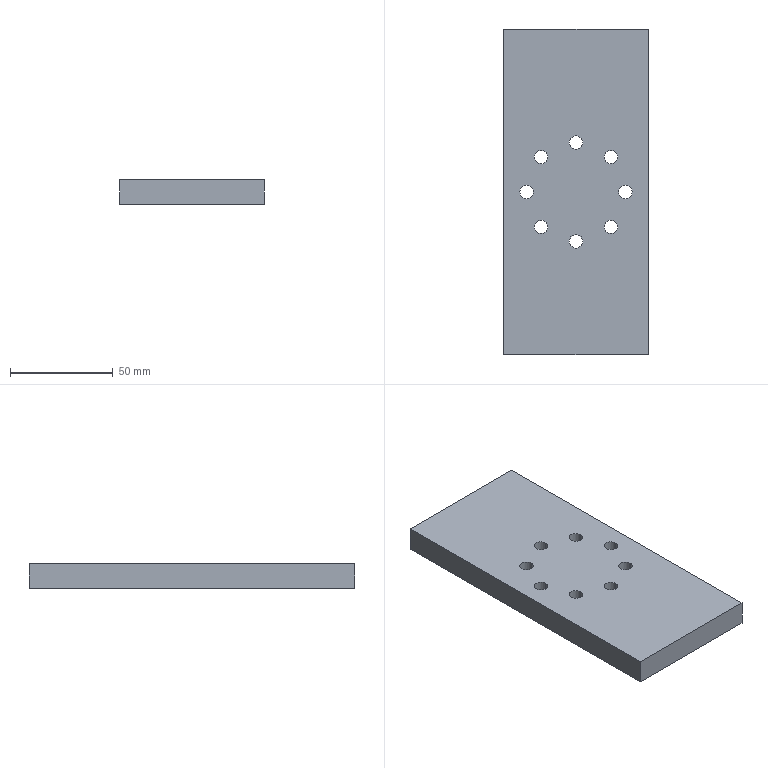Part | STEP file | Part 4^超升波生产线-2 | 1 solid | 22 faces | box 70 x 158 x 12 mm | volume 129534 mm3 | cylinder 16 | plane 6 | commonest cylinder face diameters 6.5 x16
STEP:
#1=CARTESIAN_POINT('',(-27.25,0.,12.));
#2=VERTEX_POINT('',#1);
#3=CARTESIAN_POINT('',(-20.75,0.,12.));
#4=VERTEX_POINT('',#3);
#5=CARTESIAN_POINT('',(-24.,0.,12.));
#6=DIRECTION('',(0.,0.,1.));
#7=DIRECTION('',(1.,0.,0.));
#8=AXIS2_PLACEMENT_3D('',#5,#6,#7);
#9=CIRCLE('',#8,3.25);
#10=EDGE_CURVE('',#2,#4,#9,.T.);
#11=ORIENTED_EDGE('',*,*,#10,.T.);
#12=CARTESIAN_POINT('',(-20.75,0.,0.));
#13=VERTEX_POINT('',#12);
#14=CARTESIAN_POINT('',(-20.75,0.,12.));
#15=DIRECTION('',(0.,0.,-1.));
#16=VECTOR('',#15,1000.);
#17=LINE('',#14,#16);
#18=EDGE_CURVE('',#4,#13,#17,.T.);
#19=ORIENTED_EDGE('',*,*,#18,.T.);
#20=CARTESIAN_POINT('',(-27.25,0.,0.));
#21=VERTEX_POINT('',#20);
#22=CARTESIAN_POINT('',(-24.,0.,0.));
#23=DIRECTION('',(0.,0.,1.));
#24=DIRECTION('',(1.,0.,0.));
#25=AXIS2_PLACEMENT_3D('',#22,#23,#24);
#26=CIRCLE('',#25,3.25);
#27=EDGE_CURVE('',#21,#13,#26,.T.);
#28=ORIENTED_EDGE('',*,*,#27,.F.);
#29=CARTESIAN_POINT('',(-27.25,0.,12.));
#30=DIRECTION('',(0.,0.,-1.));
#31=VECTOR('',#30,1000.);
#32=LINE('',#29,#31);
#33=EDGE_CURVE('',#2,#21,#32,.T.);
#34=ORIENTED_EDGE('',*,*,#33,.F.);
#35=EDGE_LOOP('',(#11,#19,#28,#34));
#36=FACE_OUTER_BOUND('',#35,.T.);
#37=CARTESIAN_POINT('',(-24.,0.,12.));
#38=DIRECTION('',(0.,0.,-1.));
#39=DIRECTION('',(-1.,0.,0.));
#40=AXIS2_PLACEMENT_3D('',#37,#38,#39);
#41=CYLINDRICAL_SURFACE('',#40,3.25);
#42=ADVANCED_FACE('',(#36),#41,.F.);
#43=CARTESIAN_POINT('',(-20.221,-16.971,12.));
#44=VERTEX_POINT('',#43);
#45=CARTESIAN_POINT('',(-13.721,-16.971,12.));
#46=VERTEX_POINT('',#45);
#47=CARTESIAN_POINT('',(-16.971,-16.971,12.));
#48=DIRECTION('',(0.,0.,1.));
#49=DIRECTION('',(1.,0.,0.));
#50=AXIS2_PLACEMENT_3D('',#47,#48,#49);
#51=CIRCLE('',#50,3.25);
#52=EDGE_CURVE('',#44,#46,#51,.T.);
#53=ORIENTED_EDGE('',*,*,#52,.T.);
#54=CARTESIAN_POINT('',(-13.721,-16.971,0.));
#55=VERTEX_POINT('',#54);
#56=CARTESIAN_POINT('',(-13.721,-16.971,12.));
#57=DIRECTION('',(0.,0.,-1.));
#58=VECTOR('',#57,1000.);
#59=LINE('',#56,#58);
#60=EDGE_CURVE('',#46,#55,#59,.T.);
#61=ORIENTED_EDGE('',*,*,#60,.T.);
#62=CARTESIAN_POINT('',(-20.221,-16.971,0.));
#63=VERTEX_POINT('',#62);
#64=CARTESIAN_POINT('',(-16.971,-16.971,0.));
#65=DIRECTION('',(0.,0.,1.));
#66=DIRECTION('',(1.,0.,0.));
#67=AXIS2_PLACEMENT_3D('',#64,#65,#66);
#68=CIRCLE('',#67,3.25);
#69=EDGE_CURVE('',#63,#55,#68,.T.);
#70=ORIENTED_EDGE('',*,*,#69,.F.);
#71=CARTESIAN_POINT('',(-20.221,-16.971,12.));
#72=DIRECTION('',(0.,0.,-1.));
#73=VECTOR('',#72,1000.);
#74=LINE('',#71,#73);
#75=EDGE_CURVE('',#44,#63,#74,.T.);
#76=ORIENTED_EDGE('',*,*,#75,.F.);
#77=EDGE_LOOP('',(#53,#61,#70,#76));
#78=FACE_OUTER_BOUND('',#77,.T.);
#79=CARTESIAN_POINT('',(-16.971,-16.971,12.));
#80=DIRECTION('',(0.,0.,-1.));
#81=DIRECTION('',(-1.,0.,0.));
#82=AXIS2_PLACEMENT_3D('',#79,#80,#81);
#83=CYLINDRICAL_SURFACE('',#82,3.25);
#84=ADVANCED_FACE('',(#78),#83,.F.);
#85=CARTESIAN_POINT('',(-3.25,-24.,12.));
#86=VERTEX_POINT('',#85);
#87=CARTESIAN_POINT('',(3.25,-24.,12.));
#88=VERTEX_POINT('',#87);
#89=CARTESIAN_POINT('',(0.,-24.,12.));
#90=DIRECTION('',(0.,0.,1.));
#91=DIRECTION('',(1.,0.,0.));
#92=AXIS2_PLACEMENT_3D('',#89,#90,#91);
#93=CIRCLE('',#92,3.25);
#94=EDGE_CURVE('',#86,#88,#93,.T.);
#95=ORIENTED_EDGE('',*,*,#94,.T.);
#96=CARTESIAN_POINT('',(3.25,-24.,0.));
#97=VERTEX_POINT('',#96);
#98=CARTESIAN_POINT('',(3.25,-24.,12.));
#99=DIRECTION('',(0.,0.,-1.));
#100=VECTOR('',#99,1000.);
#101=LINE('',#98,#100);
#102=EDGE_CURVE('',#88,#97,#101,.T.);
#103=ORIENTED_EDGE('',*,*,#102,.T.);
#104=CARTESIAN_POINT('',(-3.25,-24.,0.));
#105=VERTEX_POINT('',#104);
#106=CARTESIAN_POINT('',(0.,-24.,0.));
#107=DIRECTION('',(0.,0.,1.));
#108=DIRECTION('',(1.,0.,0.));
#109=AXIS2_PLACEMENT_3D('',#106,#107,#108);
#110=CIRCLE('',#109,3.25);
#111=EDGE_CURVE('',#105,#97,#110,.T.);
#112=ORIENTED_EDGE('',*,*,#111,.F.);
#113=CARTESIAN_POINT('',(-3.25,-24.,12.));
#114=DIRECTION('',(0.,0.,-1.));
#115=VECTOR('',#114,1000.);
#116=LINE('',#113,#115);
#117=EDGE_CURVE('',#86,#105,#116,.T.);
#118=ORIENTED_EDGE('',*,*,#117,.F.);
#119=EDGE_LOOP('',(#95,#103,#112,#118));
#120=FACE_OUTER_BOUND('',#119,.T.);
#121=CARTESIAN_POINT('',(0.,-24.,12.));
#122=DIRECTION('',(0.,0.,-1.));
#123=DIRECTION('',(-1.,0.,0.));
#124=AXIS2_PLACEMENT_3D('',#121,#122,#123);
#125=CYLINDRICAL_SURFACE('',#124,3.25);
#126=ADVANCED_FACE('',(#120),#125,.F.);
#127=CARTESIAN_POINT('',(13.721,-16.971,12.));
#128=VERTEX_POINT('',#127);
#129=CARTESIAN_POINT('',(20.221,-16.971,12.));
#130=VERTEX_POINT('',#129);
#131=CARTESIAN_POINT('',(16.971,-16.971,12.));
#132=DIRECTION('',(0.,0.,1.));
#133=DIRECTION('',(1.,0.,0.));
#134=AXIS2_PLACEMENT_3D('',#131,#132,#133);
#135=CIRCLE('',#134,3.25);
#136=EDGE_CURVE('',#128,#130,#135,.T.);
#137=ORIENTED_EDGE('',*,*,#136,.T.);
#138=CARTESIAN_POINT('',(20.221,-16.971,0.));
#139=VERTEX_POINT('',#138);
#140=CARTESIAN_POINT('',(20.221,-16.971,12.));
#141=DIRECTION('',(0.,0.,-1.));
#142=VECTOR('',#141,1000.);
#143=LINE('',#140,#142);
#144=EDGE_CURVE('',#130,#139,#143,.T.);
#145=ORIENTED_EDGE('',*,*,#144,.T.);
#146=CARTESIAN_POINT('',(13.721,-16.971,0.));
#147=VERTEX_POINT('',#146);
#148=CARTESIAN_POINT('',(16.971,-16.971,0.));
#149=DIRECTION('',(0.,0.,1.));
#150=DIRECTION('',(1.,0.,0.));
#151=AXIS2_PLACEMENT_3D('',#148,#149,#150);
#152=CIRCLE('',#151,3.25);
#153=EDGE_CURVE('',#147,#139,#152,.T.);
#154=ORIENTED_EDGE('',*,*,#153,.F.);
#155=CARTESIAN_POINT('',(13.721,-16.971,12.));
#156=DIRECTION('',(0.,0.,-1.));
#157=VECTOR('',#156,1000.);
#158=LINE('',#155,#157);
#159=EDGE_CURVE('',#128,#147,#158,.T.);
#160=ORIENTED_EDGE('',*,*,#159,.F.);
#161=EDGE_LOOP('',(#137,#145,#154,#160));
#162=FACE_OUTER_BOUND('',#161,.T.);
#163=CARTESIAN_POINT('',(16.971,-16.971,12.));
#164=DIRECTION('',(0.,0.,-1.));
#165=DIRECTION('',(-1.,0.,0.));
#166=AXIS2_PLACEMENT_3D('',#163,#164,#165);
#167=CYLINDRICAL_SURFACE('',#166,3.25);
#168=ADVANCED_FACE('',(#162),#167,.F.);
#169=CARTESIAN_POINT('',(20.75,0.,12.));
#170=VERTEX_POINT('',#169);
#171=CARTESIAN_POINT('',(27.25,0.,12.));
#172=VERTEX_POINT('',#171);
#173=CARTESIAN_POINT('',(24.,0.,12.));
#174=DIRECTION('',(0.,0.,1.));
#175=DIRECTION('',(1.,0.,0.));
#176=AXIS2_PLACEMENT_3D('',#173,#174,#175);
#177=CIRCLE('',#176,3.25);
#178=EDGE_CURVE('',#170,#172,#177,.T.);
#179=ORIENTED_EDGE('',*,*,#178,.T.);
#180=CARTESIAN_POINT('',(27.25,0.,0.));
#181=VERTEX_POINT('',#180);
#182=CARTESIAN_POINT('',(27.25,0.,12.));
#183=DIRECTION('',(0.,0.,-1.));
#184=VECTOR('',#183,1000.);
#185=LINE('',#182,#184);
#186=EDGE_CURVE('',#172,#181,#185,.T.);
#187=ORIENTED_EDGE('',*,*,#186,.T.);
#188=CARTESIAN_POINT('',(20.75,0.,0.));
#189=VERTEX_POINT('',#188);
#190=CARTESIAN_POINT('',(24.,0.,0.));
#191=DIRECTION('',(0.,0.,1.));
#192=DIRECTION('',(1.,0.,0.));
#193=AXIS2_PLACEMENT_3D('',#190,#191,#192);
#194=CIRCLE('',#193,3.25);
#195=EDGE_CURVE('',#189,#181,#194,.T.);
#196=ORIENTED_EDGE('',*,*,#195,.F.);
#197=CARTESIAN_POINT('',(20.75,0.,12.));
#198=DIRECTION('',(0.,0.,-1.));
#199=VECTOR('',#198,1000.);
#200=LINE('',#197,#199);
#201=EDGE_CURVE('',#170,#189,#200,.T.);
#202=ORIENTED_EDGE('',*,*,#201,.F.);
#203=EDGE_LOOP('',(#179,#187,#196,#202));
#204=FACE_OUTER_BOUND('',#203,.T.);
#205=CARTESIAN_POINT('',(24.,0.,12.));
#206=DIRECTION('',(0.,0.,-1.));
#207=DIRECTION('',(-1.,0.,0.));
#208=AXIS2_PLACEMENT_3D('',#205,#206,#207);
#209=CYLINDRICAL_SURFACE('',#208,3.25);
#210=ADVANCED_FACE('',(#204),#209,.F.);
#211=CARTESIAN_POINT('',(13.721,16.971,12.));
#212=VERTEX_POINT('',#211);
#213=CARTESIAN_POINT('',(20.221,16.971,12.));
#214=VERTEX_POINT('',#213);
#215=CARTESIAN_POINT('',(16.971,16.971,12.));
#216=DIRECTION('',(0.,0.,1.));
#217=DIRECTION('',(1.,0.,0.));
#218=AXIS2_PLACEMENT_3D('',#215,#216,#217);
#219=CIRCLE('',#218,3.25);
#220=EDGE_CURVE('',#212,#214,#219,.T.);
#221=ORIENTED_EDGE('',*,*,#220,.T.);
#222=CARTESIAN_POINT('',(20.221,16.971,0.));
#223=VERTEX_POINT('',#222);
#224=CARTESIAN_POINT('',(20.221,16.971,12.));
#225=DIRECTION('',(0.,0.,-1.));
#226=VECTOR('',#225,1000.);
#227=LINE('',#224,#226);
#228=EDGE_CURVE('',#214,#223,#227,.T.);
#229=ORIENTED_EDGE('',*,*,#228,.T.);
#230=CARTESIAN_POINT('',(13.721,16.971,0.));
#231=VERTEX_POINT('',#230);
#232=CARTESIAN_POINT('',(16.971,16.971,0.));
#233=DIRECTION('',(0.,0.,1.));
#234=DIRECTION('',(1.,0.,0.));
#235=AXIS2_PLACEMENT_3D('',#232,#233,#234);
#236=CIRCLE('',#235,3.25);
#237=EDGE_CURVE('',#231,#223,#236,.T.);
#238=ORIENTED_EDGE('',*,*,#237,.F.);
#239=CARTESIAN_POINT('',(13.721,16.971,12.));
#240=DIRECTION('',(0.,0.,-1.));
#241=VECTOR('',#240,1000.);
#242=LINE('',#239,#241);
#243=EDGE_CURVE('',#212,#231,#242,.T.);
#244=ORIENTED_EDGE('',*,*,#243,.F.);
#245=EDGE_LOOP('',(#221,#229,#238,#244));
#246=FACE_OUTER_BOUND('',#245,.T.);
#247=CARTESIAN_POINT('',(16.971,16.971,12.));
#248=DIRECTION('',(0.,0.,-1.));
#249=DIRECTION('',(-1.,0.,0.));
#250=AXIS2_PLACEMENT_3D('',#247,#248,#249);
#251=CYLINDRICAL_SURFACE('',#250,3.25);
#252=ADVANCED_FACE('',(#246),#251,.F.);
#253=CARTESIAN_POINT('',(-3.25,24.,12.));
#254=VERTEX_POINT('',#253);
#255=CARTESIAN_POINT('',(3.25,24.,12.));
#256=VERTEX_POINT('',#255);
#257=CARTESIAN_POINT('',(0.,24.,12.));
#258=DIRECTION('',(0.,0.,1.));
#259=DIRECTION('',(1.,0.,0.));
#260=AXIS2_PLACEMENT_3D('',#257,#258,#259);
#261=CIRCLE('',#260,3.25);
#262=EDGE_CURVE('',#254,#256,#261,.T.);
#263=ORIENTED_EDGE('',*,*,#262,.T.);
#264=CARTESIAN_POINT('',(3.25,24.,0.));
#265=VERTEX_POINT('',#264);
#266=CARTESIAN_POINT('',(3.25,24.,12.));
#267=DIRECTION('',(0.,0.,-1.));
#268=VECTOR('',#267,1000.);
#269=LINE('',#266,#268);
#270=EDGE_CURVE('',#256,#265,#269,.T.);
#271=ORIENTED_EDGE('',*,*,#270,.T.);
#272=CARTESIAN_POINT('',(-3.25,24.,0.));
#273=VERTEX_POINT('',#272);
#274=CARTESIAN_POINT('',(0.,24.,0.));
#275=DIRECTION('',(0.,0.,1.));
#276=DIRECTION('',(1.,0.,0.));
#277=AXIS2_PLACEMENT_3D('',#274,#275,#276);
#278=CIRCLE('',#277,3.25);
#279=EDGE_CURVE('',#273,#265,#278,.T.);
#280=ORIENTED_EDGE('',*,*,#279,.F.);
#281=CARTESIAN_POINT('',(-3.25,24.,12.));
#282=DIRECTION('',(0.,0.,-1.));
#283=VECTOR('',#282,1000.);
#284=LINE('',#281,#283);
#285=EDGE_CURVE('',#254,#273,#284,.T.);
#286=ORIENTED_EDGE('',*,*,#285,.F.);
#287=EDGE_LOOP('',(#263,#271,#280,#286));
#288=FACE_OUTER_BOUND('',#287,.T.);
#289=CARTESIAN_POINT('',(0.,24.,12.));
#290=DIRECTION('',(0.,0.,-1.));
#291=DIRECTION('',(-1.,0.,0.));
#292=AXIS2_PLACEMENT_3D('',#289,#290,#291);
#293=CYLINDRICAL_SURFACE('',#292,3.25);
#294=ADVANCED_FACE('',(#288),#293,.F.);
#295=CARTESIAN_POINT('',(-20.221,16.971,12.));
#296=VERTEX_POINT('',#295);
#297=CARTESIAN_POINT('',(-13.721,16.971,12.));
#298=VERTEX_POINT('',#297);
#299=CARTESIAN_POINT('',(-16.971,16.971,12.));
#300=DIRECTION('',(0.,0.,1.));
#301=DIRECTION('',(1.,0.,0.));
#302=AXIS2_PLACEMENT_3D('',#299,#300,#301);
#303=CIRCLE('',#302,3.25);
#304=EDGE_CURVE('',#296,#298,#303,.T.);
#305=ORIENTED_EDGE('',*,*,#304,.T.);
#306=CARTESIAN_POINT('',(-13.721,16.971,0.));
#307=VERTEX_POINT('',#306);
#308=CARTESIAN_POINT('',(-13.721,16.971,12.));
#309=DIRECTION('',(0.,0.,-1.));
#310=VECTOR('',#309,1000.);
#311=LINE('',#308,#310);
#312=EDGE_CURVE('',#298,#307,#311,.T.);
#313=ORIENTED_EDGE('',*,*,#312,.T.);
#314=CARTESIAN_POINT('',(-20.221,16.971,0.));
#315=VERTEX_POINT('',#314);
#316=CARTESIAN_POINT('',(-16.971,16.971,0.));
#317=DIRECTION('',(0.,0.,1.));
#318=DIRECTION('',(1.,0.,0.));
#319=AXIS2_PLACEMENT_3D('',#316,#317,#318);
#320=CIRCLE('',#319,3.25);
#321=EDGE_CURVE('',#315,#307,#320,.T.);
#322=ORIENTED_EDGE('',*,*,#321,.F.);
#323=CARTESIAN_POINT('',(-20.221,16.971,12.));
#324=DIRECTION('',(0.,0.,-1.));
#325=VECTOR('',#324,1000.);
#326=LINE('',#323,#325);
#327=EDGE_CURVE('',#296,#315,#326,.T.);
#328=ORIENTED_EDGE('',*,*,#327,.F.);
#329=EDGE_LOOP('',(#305,#313,#322,#328));
#330=FACE_OUTER_BOUND('',#329,.T.);
#331=CARTESIAN_POINT('',(-16.971,16.971,12.));
#332=DIRECTION('',(0.,0.,-1.));
#333=DIRECTION('',(-1.,0.,0.));
#334=AXIS2_PLACEMENT_3D('',#331,#332,#333);
#335=CYLINDRICAL_SURFACE('',#334,3.25);
#336=ADVANCED_FACE('',(#330),#335,.F.);
#337=ORIENTED_EDGE('',*,*,#52,.F.);
#338=CARTESIAN_POINT('',(-16.971,-16.971,12.));
#339=DIRECTION('',(0.,0.,1.));
#340=DIRECTION('',(1.,0.,0.));
#341=AXIS2_PLACEMENT_3D('',#338,#339,#340);
#342=CIRCLE('',#341,3.25);
#343=EDGE_CURVE('',#46,#44,#342,.T.);
#344=ORIENTED_EDGE('',*,*,#343,.F.);
#345=EDGE_LOOP('',(#337,#344));
#346=FACE_BOUND('',#345,.T.);
#347=ORIENTED_EDGE('',*,*,#136,.F.);
#348=CARTESIAN_POINT('',(16.971,-16.971,12.));
#349=DIRECTION('',(0.,0.,1.));
#350=DIRECTION('',(1.,0.,0.));
#351=AXIS2_PLACEMENT_3D('',#348,#349,#350);
#352=CIRCLE('',#351,3.25);
#353=EDGE_CURVE('',#130,#128,#352,.T.);
#354=ORIENTED_EDGE('',*,*,#353,.F.);
#355=EDGE_LOOP('',(#347,#354));
#356=FACE_BOUND('',#355,.T.);
#357=ORIENTED_EDGE('',*,*,#220,.F.);
#358=CARTESIAN_POINT('',(16.971,16.971,12.));
#359=DIRECTION('',(0.,0.,1.));
#360=DIRECTION('',(1.,0.,0.));
#361=AXIS2_PLACEMENT_3D('',#358,#359,#360);
#362=CIRCLE('',#361,3.25);
#363=EDGE_CURVE('',#214,#212,#362,.T.);
#364=ORIENTED_EDGE('',*,*,#363,.F.);
#365=EDGE_LOOP('',(#357,#364));
#366=FACE_BOUND('',#365,.T.);
#367=ORIENTED_EDGE('',*,*,#304,.F.);
#368=CARTESIAN_POINT('',(-16.971,16.971,12.));
#369=DIRECTION('',(0.,0.,1.));
#370=DIRECTION('',(1.,0.,0.));
#371=AXIS2_PLACEMENT_3D('',#368,#369,#370);
#372=CIRCLE('',#371,3.25);
#373=EDGE_CURVE('',#298,#296,#372,.T.);
#374=ORIENTED_EDGE('',*,*,#373,.F.);
#375=EDGE_LOOP('',(#367,#374));
#376=FACE_BOUND('',#375,.T.);
#377=CARTESIAN_POINT('',(35.,-79.,12.));
#378=VERTEX_POINT('',#377);
#379=CARTESIAN_POINT('',(35.,79.,12.));
#380=VERTEX_POINT('',#379);
#381=CARTESIAN_POINT('',(35.,79.,12.));
#382=DIRECTION('',(0.,1.,0.));
#383=VECTOR('',#382,1000.);
#384=LINE('',#381,#383);
#385=EDGE_CURVE('',#378,#380,#384,.T.);
#386=ORIENTED_EDGE('',*,*,#385,.T.);
#387=CARTESIAN_POINT('',(-35.,79.,12.));
#388=VERTEX_POINT('',#387);
#389=CARTESIAN_POINT('',(-35.,79.,12.));
#390=DIRECTION('',(-1.,0.,0.));
#391=VECTOR('',#390,1000.);
#392=LINE('',#389,#391);
#393=EDGE_CURVE('',#380,#388,#392,.T.);
#394=ORIENTED_EDGE('',*,*,#393,.T.);
#395=CARTESIAN_POINT('',(-35.,-79.,12.));
#396=VERTEX_POINT('',#395);
#397=CARTESIAN_POINT('',(-35.,79.,12.));
#398=DIRECTION('',(0.,-1.,0.));
#399=VECTOR('',#398,1000.);
#400=LINE('',#397,#399);
#401=EDGE_CURVE('',#388,#396,#400,.T.);
#402=ORIENTED_EDGE('',*,*,#401,.T.);
#403=CARTESIAN_POINT('',(-35.,-79.,12.));
#404=DIRECTION('',(1.,0.,0.));
#405=VECTOR('',#404,1000.);
#406=LINE('',#403,#405);
#407=EDGE_CURVE('',#396,#378,#406,.T.);
#408=ORIENTED_EDGE('',*,*,#407,.T.);
#409=EDGE_LOOP('',(#386,#394,#402,#408));
#410=FACE_OUTER_BOUND('',#409,.T.);
#411=ORIENTED_EDGE('',*,*,#262,.F.);
#412=CARTESIAN_POINT('',(0.,24.,12.));
#413=DIRECTION('',(0.,0.,1.));
#414=DIRECTION('',(1.,0.,0.));
#415=AXIS2_PLACEMENT_3D('',#412,#413,#414);
#416=CIRCLE('',#415,3.25);
#417=EDGE_CURVE('',#256,#254,#416,.T.);
#418=ORIENTED_EDGE('',*,*,#417,.F.);
#419=EDGE_LOOP('',(#411,#418));
#420=FACE_BOUND('',#419,.T.);
#421=ORIENTED_EDGE('',*,*,#178,.F.);
#422=CARTESIAN_POINT('',(24.,0.,12.));
#423=DIRECTION('',(0.,0.,1.));
#424=DIRECTION('',(1.,0.,0.));
#425=AXIS2_PLACEMENT_3D('',#422,#423,#424);
#426=CIRCLE('',#425,3.25);
#427=EDGE_CURVE('',#172,#170,#426,.T.);
#428=ORIENTED_EDGE('',*,*,#427,.F.);
#429=EDGE_LOOP('',(#421,#428));
#430=FACE_BOUND('',#429,.T.);
#431=ORIENTED_EDGE('',*,*,#94,.F.);
#432=CARTESIAN_POINT('',(0.,-24.,12.));
#433=DIRECTION('',(0.,0.,1.));
#434=DIRECTION('',(1.,0.,0.));
#435=AXIS2_PLACEMENT_3D('',#432,#433,#434);
#436=CIRCLE('',#435,3.25);
#437=EDGE_CURVE('',#88,#86,#436,.T.);
#438=ORIENTED_EDGE('',*,*,#437,.F.);
#439=EDGE_LOOP('',(#431,#438));
#440=FACE_BOUND('',#439,.T.);
#441=ORIENTED_EDGE('',*,*,#10,.F.);
#442=CARTESIAN_POINT('',(-24.,0.,12.));
#443=DIRECTION('',(0.,0.,1.));
#444=DIRECTION('',(1.,0.,0.));
#445=AXIS2_PLACEMENT_3D('',#442,#443,#444);
#446=CIRCLE('',#445,3.25);
#447=EDGE_CURVE('',#4,#2,#446,.T.);
#448=ORIENTED_EDGE('',*,*,#447,.F.);
#449=EDGE_LOOP('',(#441,#448));
#450=FACE_BOUND('',#449,.T.);
#451=CARTESIAN_POINT('',(35.,-79.,12.));
#452=DIRECTION('',(0.,0.,1.));
#453=DIRECTION('',(1.,0.,0.));
#454=AXIS2_PLACEMENT_3D('',#451,#452,#453);
#455=PLANE('',#454);
#456=ADVANCED_FACE('',(#346,#356,#366,#376,#410,#420,#430,#440,#450),#455,.T.);
#457=ORIENTED_EDGE('',*,*,#69,.T.);
#458=CARTESIAN_POINT('',(-16.971,-16.971,0.));
#459=DIRECTION('',(0.,0.,1.));
#460=DIRECTION('',(1.,0.,0.));
#461=AXIS2_PLACEMENT_3D('',#458,#459,#460);
#462=CIRCLE('',#461,3.25);
#463=EDGE_CURVE('',#55,#63,#462,.T.);
#464=ORIENTED_EDGE('',*,*,#463,.T.);
#465=EDGE_LOOP('',(#457,#464));
#466=FACE_BOUND('',#465,.T.);
#467=ORIENTED_EDGE('',*,*,#153,.T.);
#468=CARTESIAN_POINT('',(16.971,-16.971,0.));
#469=DIRECTION('',(0.,0.,1.));
#470=DIRECTION('',(1.,0.,0.));
#471=AXIS2_PLACEMENT_3D('',#468,#469,#470);
#472=CIRCLE('',#471,3.25);
#473=EDGE_CURVE('',#139,#147,#472,.T.);
#474=ORIENTED_EDGE('',*,*,#473,.T.);
#475=EDGE_LOOP('',(#467,#474));
#476=FACE_BOUND('',#475,.T.);
#477=ORIENTED_EDGE('',*,*,#237,.T.);
#478=CARTESIAN_POINT('',(16.971,16.971,0.));
#479=DIRECTION('',(0.,0.,1.));
#480=DIRECTION('',(1.,0.,0.));
#481=AXIS2_PLACEMENT_3D('',#478,#479,#480);
#482=CIRCLE('',#481,3.25);
#483=EDGE_CURVE('',#223,#231,#482,.T.);
#484=ORIENTED_EDGE('',*,*,#483,.T.);
#485=EDGE_LOOP('',(#477,#484));
#486=FACE_BOUND('',#485,.T.);
#487=ORIENTED_EDGE('',*,*,#321,.T.);
#488=CARTESIAN_POINT('',(-16.971,16.971,0.));
#489=DIRECTION('',(0.,0.,1.));
#490=DIRECTION('',(1.,0.,0.));
#491=AXIS2_PLACEMENT_3D('',#488,#489,#490);
#492=CIRCLE('',#491,3.25);
#493=EDGE_CURVE('',#307,#315,#492,.T.);
#494=ORIENTED_EDGE('',*,*,#493,.T.);
#495=EDGE_LOOP('',(#487,#494));
#496=FACE_BOUND('',#495,.T.);
#497=CARTESIAN_POINT('',(35.,-79.,0.));
#498=VERTEX_POINT('',#497);
#499=CARTESIAN_POINT('',(35.,79.,0.));
#500=VERTEX_POINT('',#499);
#501=CARTESIAN_POINT('',(35.,79.,0.));
#502=DIRECTION('',(0.,1.,0.));
#503=VECTOR('',#502,1000.);
#504=LINE('',#501,#503);
#505=EDGE_CURVE('',#498,#500,#504,.T.);
#506=ORIENTED_EDGE('',*,*,#505,.F.);
#507=CARTESIAN_POINT('',(-35.,-79.,0.));
#508=VERTEX_POINT('',#507);
#509=CARTESIAN_POINT('',(-35.,-79.,0.));
#510=DIRECTION('',(1.,0.,0.));
#511=VECTOR('',#510,1000.);
#512=LINE('',#509,#511);
#513=EDGE_CURVE('',#508,#498,#512,.T.);
#514=ORIENTED_EDGE('',*,*,#513,.F.);
#515=CARTESIAN_POINT('',(-35.,79.,0.));
#516=VERTEX_POINT('',#515);
#517=CARTESIAN_POINT('',(-35.,79.,0.));
#518=DIRECTION('',(0.,-1.,0.));
#519=VECTOR('',#518,1000.);
#520=LINE('',#517,#519);
#521=EDGE_CURVE('',#516,#508,#520,.T.);
#522=ORIENTED_EDGE('',*,*,#521,.F.);
#523=CARTESIAN_POINT('',(-35.,79.,0.));
#524=DIRECTION('',(-1.,0.,0.));
#525=VECTOR('',#524,1000.);
#526=LINE('',#523,#525);
#527=EDGE_CURVE('',#500,#516,#526,.T.);
#528=ORIENTED_EDGE('',*,*,#527,.F.);
#529=EDGE_LOOP('',(#506,#514,#522,#528));
#530=FACE_OUTER_BOUND('',#529,.T.);
#531=ORIENTED_EDGE('',*,*,#279,.T.);
#532=CARTESIAN_POINT('',(0.,24.,0.));
#533=DIRECTION('',(0.,0.,1.));
#534=DIRECTION('',(1.,0.,0.));
#535=AXIS2_PLACEMENT_3D('',#532,#533,#534);
#536=CIRCLE('',#535,3.25);
#537=EDGE_CURVE('',#265,#273,#536,.T.);
#538=ORIENTED_EDGE('',*,*,#537,.T.);
#539=EDGE_LOOP('',(#531,#538));
#540=FACE_BOUND('',#539,.T.);
#541=ORIENTED_EDGE('',*,*,#195,.T.);
#542=CARTESIAN_POINT('',(24.,0.,0.));
#543=DIRECTION('',(0.,0.,1.));
#544=DIRECTION('',(1.,0.,0.));
#545=AXIS2_PLACEMENT_3D('',#542,#543,#544);
#546=CIRCLE('',#545,3.25);
#547=EDGE_CURVE('',#181,#189,#546,.T.);
#548=ORIENTED_EDGE('',*,*,#547,.T.);
#549=EDGE_LOOP('',(#541,#548));
#550=FACE_BOUND('',#549,.T.);
#551=ORIENTED_EDGE('',*,*,#111,.T.);
#552=CARTESIAN_POINT('',(0.,-24.,0.));
#553=DIRECTION('',(0.,0.,1.));
#554=DIRECTION('',(1.,0.,0.));
#555=AXIS2_PLACEMENT_3D('',#552,#553,#554);
#556=CIRCLE('',#555,3.25);
#557=EDGE_CURVE('',#97,#105,#556,.T.);
#558=ORIENTED_EDGE('',*,*,#557,.T.);
#559=EDGE_LOOP('',(#551,#558));
#560=FACE_BOUND('',#559,.T.);
#561=ORIENTED_EDGE('',*,*,#27,.T.);
#562=CARTESIAN_POINT('',(-24.,0.,0.));
#563=DIRECTION('',(0.,0.,1.));
#564=DIRECTION('',(1.,0.,0.));
#565=AXIS2_PLACEMENT_3D('',#562,#563,#564);
#566=CIRCLE('',#565,3.25);
#567=EDGE_CURVE('',#13,#21,#566,.T.);
#568=ORIENTED_EDGE('',*,*,#567,.T.);
#569=EDGE_LOOP('',(#561,#568));
#570=FACE_BOUND('',#569,.T.);
#571=CARTESIAN_POINT('',(35.,-79.,0.));
#572=DIRECTION('',(0.,0.,1.));
#573=DIRECTION('',(1.,0.,0.));
#574=AXIS2_PLACEMENT_3D('',#571,#572,#573);
#575=PLANE('',#574);
#576=ADVANCED_FACE('',(#466,#476,#486,#496,#530,#540,#550,#560,#570),#575,.F.);
#577=ORIENTED_EDGE('',*,*,#505,.T.);
#578=CARTESIAN_POINT('',(35.,79.,12.));
#579=DIRECTION('',(0.,0.,-1.));
#580=VECTOR('',#579,1000.);
#581=LINE('',#578,#580);
#582=EDGE_CURVE('',#380,#500,#581,.T.);
#583=ORIENTED_EDGE('',*,*,#582,.F.);
#584=ORIENTED_EDGE('',*,*,#385,.F.);
#585=CARTESIAN_POINT('',(35.,-79.,12.));
#586=DIRECTION('',(0.,0.,-1.));
#587=VECTOR('',#586,1000.);
#588=LINE('',#585,#587);
#589=EDGE_CURVE('',#378,#498,#588,.T.);
#590=ORIENTED_EDGE('',*,*,#589,.T.);
#591=EDGE_LOOP('',(#577,#583,#584,#590));
#592=FACE_OUTER_BOUND('',#591,.T.);
#593=CARTESIAN_POINT('',(35.,79.,12.));
#594=DIRECTION('',(-1.,0.,0.));
#595=DIRECTION('',(0.,-1.,0.));
#596=AXIS2_PLACEMENT_3D('',#593,#594,#595);
#597=PLANE('',#596);
#598=ADVANCED_FACE('',(#592),#597,.F.);
#599=ORIENTED_EDGE('',*,*,#527,.T.);
#600=CARTESIAN_POINT('',(-35.,79.,12.));
#601=DIRECTION('',(0.,0.,-1.));
#602=VECTOR('',#601,1000.);
#603=LINE('',#600,#602);
#604=EDGE_CURVE('',#388,#516,#603,.T.);
#605=ORIENTED_EDGE('',*,*,#604,.F.);
#606=ORIENTED_EDGE('',*,*,#393,.F.);
#607=ORIENTED_EDGE('',*,*,#582,.T.);
#608=EDGE_LOOP('',(#599,#605,#606,#607));
#609=FACE_OUTER_BOUND('',#608,.T.);
#610=CARTESIAN_POINT('',(-35.,79.,12.));
#611=DIRECTION('',(0.,-1.,0.));
#612=DIRECTION('',(0.,0.,-1.));
#613=AXIS2_PLACEMENT_3D('',#610,#611,#612);
#614=PLANE('',#613);
#615=ADVANCED_FACE('',(#609),#614,.F.);
#616=ORIENTED_EDGE('',*,*,#521,.T.);
#617=CARTESIAN_POINT('',(-35.,-79.,12.));
#618=DIRECTION('',(0.,0.,-1.));
#619=VECTOR('',#618,1000.);
#620=LINE('',#617,#619);
#621=EDGE_CURVE('',#396,#508,#620,.T.);
#622=ORIENTED_EDGE('',*,*,#621,.F.);
#623=ORIENTED_EDGE('',*,*,#401,.F.);
#624=ORIENTED_EDGE('',*,*,#604,.T.);
#625=EDGE_LOOP('',(#616,#622,#623,#624));
#626=FACE_OUTER_BOUND('',#625,.T.);
#627=CARTESIAN_POINT('',(-35.,79.,12.));
#628=DIRECTION('',(1.,0.,0.));
#629=DIRECTION('',(0.,1.,0.));
#630=AXIS2_PLACEMENT_3D('',#627,#628,#629);
#631=PLANE('',#630);
#632=ADVANCED_FACE('',(#626),#631,.F.);
#633=ORIENTED_EDGE('',*,*,#513,.T.);
#634=ORIENTED_EDGE('',*,*,#589,.F.);
#635=ORIENTED_EDGE('',*,*,#407,.F.);
#636=ORIENTED_EDGE('',*,*,#621,.T.);
#637=EDGE_LOOP('',(#633,#634,#635,#636));
#638=FACE_OUTER_BOUND('',#637,.T.);
#639=CARTESIAN_POINT('',(-35.,-79.,12.));
#640=DIRECTION('',(0.,1.,0.));
#641=DIRECTION('',(0.,0.,1.));
#642=AXIS2_PLACEMENT_3D('',#639,#640,#641);
#643=PLANE('',#642);
#644=ADVANCED_FACE('',(#638),#643,.F.);
#645=ORIENTED_EDGE('',*,*,#312,.F.);
#646=ORIENTED_EDGE('',*,*,#373,.T.);
#647=ORIENTED_EDGE('',*,*,#327,.T.);
#648=ORIENTED_EDGE('',*,*,#493,.F.);
#649=EDGE_LOOP('',(#645,#646,#647,#648));
#650=FACE_OUTER_BOUND('',#649,.T.);
#651=CARTESIAN_POINT('',(-16.971,16.971,12.));
#652=DIRECTION('',(0.,0.,-1.));
#653=DIRECTION('',(-1.,0.,0.));
#654=AXIS2_PLACEMENT_3D('',#651,#652,#653);
#655=CYLINDRICAL_SURFACE('',#654,3.25);
#656=ADVANCED_FACE('',(#650),#655,.F.);
#657=ORIENTED_EDGE('',*,*,#270,.F.);
#658=ORIENTED_EDGE('',*,*,#417,.T.);
#659=ORIENTED_EDGE('',*,*,#285,.T.);
#660=ORIENTED_EDGE('',*,*,#537,.F.);
#661=EDGE_LOOP('',(#657,#658,#659,#660));
#662=FACE_OUTER_BOUND('',#661,.T.);
#663=CARTESIAN_POINT('',(0.,24.,12.));
#664=DIRECTION('',(0.,0.,-1.));
#665=DIRECTION('',(-1.,0.,0.));
#666=AXIS2_PLACEMENT_3D('',#663,#664,#665);
#667=CYLINDRICAL_SURFACE('',#666,3.25);
#668=ADVANCED_FACE('',(#662),#667,.F.);
#669=ORIENTED_EDGE('',*,*,#228,.F.);
#670=ORIENTED_EDGE('',*,*,#363,.T.);
#671=ORIENTED_EDGE('',*,*,#243,.T.);
#672=ORIENTED_EDGE('',*,*,#483,.F.);
#673=EDGE_LOOP('',(#669,#670,#671,#672));
#674=FACE_OUTER_BOUND('',#673,.T.);
#675=CARTESIAN_POINT('',(16.971,16.971,12.));
#676=DIRECTION('',(0.,0.,-1.));
#677=DIRECTION('',(-1.,0.,0.));
#678=AXIS2_PLACEMENT_3D('',#675,#676,#677);
#679=CYLINDRICAL_SURFACE('',#678,3.25);
#680=ADVANCED_FACE('',(#674),#679,.F.);
#681=ORIENTED_EDGE('',*,*,#186,.F.);
#682=ORIENTED_EDGE('',*,*,#427,.T.);
#683=ORIENTED_EDGE('',*,*,#201,.T.);
#684=ORIENTED_EDGE('',*,*,#547,.F.);
#685=EDGE_LOOP('',(#681,#682,#683,#684));
#686=FACE_OUTER_BOUND('',#685,.T.);
#687=CARTESIAN_POINT('',(24.,0.,12.));
#688=DIRECTION('',(0.,0.,-1.));
#689=DIRECTION('',(-1.,0.,0.));
#690=AXIS2_PLACEMENT_3D('',#687,#688,#689);
#691=CYLINDRICAL_SURFACE('',#690,3.25);
#692=ADVANCED_FACE('',(#686),#691,.F.);
#693=ORIENTED_EDGE('',*,*,#144,.F.);
#694=ORIENTED_EDGE('',*,*,#353,.T.);
#695=ORIENTED_EDGE('',*,*,#159,.T.);
#696=ORIENTED_EDGE('',*,*,#473,.F.);
#697=EDGE_LOOP('',(#693,#694,#695,#696));
#698=FACE_OUTER_BOUND('',#697,.T.);
#699=CARTESIAN_POINT('',(16.971,-16.971,12.));
#700=DIRECTION('',(0.,0.,-1.));
#701=DIRECTION('',(-1.,0.,0.));
#702=AXIS2_PLACEMENT_3D('',#699,#700,#701);
#703=CYLINDRICAL_SURFACE('',#702,3.25);
#704=ADVANCED_FACE('',(#698),#703,.F.);
#705=ORIENTED_EDGE('',*,*,#102,.F.);
#706=ORIENTED_EDGE('',*,*,#437,.T.);
#707=ORIENTED_EDGE('',*,*,#117,.T.);
#708=ORIENTED_EDGE('',*,*,#557,.F.);
#709=EDGE_LOOP('',(#705,#706,#707,#708));
#710=FACE_OUTER_BOUND('',#709,.T.);
#711=CARTESIAN_POINT('',(0.,-24.,12.));
#712=DIRECTION('',(0.,0.,-1.));
#713=DIRECTION('',(-1.,0.,0.));
#714=AXIS2_PLACEMENT_3D('',#711,#712,#713);
#715=CYLINDRICAL_SURFACE('',#714,3.25);
#716=ADVANCED_FACE('',(#710),#715,.F.);
#717=ORIENTED_EDGE('',*,*,#60,.F.);
#718=ORIENTED_EDGE('',*,*,#343,.T.);
#719=ORIENTED_EDGE('',*,*,#75,.T.);
#720=ORIENTED_EDGE('',*,*,#463,.F.);
#721=EDGE_LOOP('',(#717,#718,#719,#720));
#722=FACE_OUTER_BOUND('',#721,.T.);
#723=CARTESIAN_POINT('',(-16.971,-16.971,12.));
#724=DIRECTION('',(0.,0.,-1.));
#725=DIRECTION('',(-1.,0.,0.));
#726=AXIS2_PLACEMENT_3D('',#723,#724,#725);
#727=CYLINDRICAL_SURFACE('',#726,3.25);
#728=ADVANCED_FACE('',(#722),#727,.F.);
#729=ORIENTED_EDGE('',*,*,#18,.F.);
#730=ORIENTED_EDGE('',*,*,#447,.T.);
#731=ORIENTED_EDGE('',*,*,#33,.T.);
#732=ORIENTED_EDGE('',*,*,#567,.F.);
#733=EDGE_LOOP('',(#729,#730,#731,#732));
#734=FACE_OUTER_BOUND('',#733,.T.);
#735=CARTESIAN_POINT('',(-24.,0.,12.));
#736=DIRECTION('',(0.,0.,-1.));
#737=DIRECTION('',(-1.,0.,0.));
#738=AXIS2_PLACEMENT_3D('',#735,#736,#737);
#739=CYLINDRICAL_SURFACE('',#738,3.25);
#740=ADVANCED_FACE('',(#734),#739,.F.);
#741=CLOSED_SHELL('',(#42,#84,#126,#168,#210,#252,#294,#336,#456,#576,#598,#615,#632,#644,#656,#668,#680,#692,#704,#716,#728,#740));
#742=MANIFOLD_SOLID_BREP('',#741);
#743=CARTESIAN_POINT('',(0.,0.,0.));
#744=DIRECTION('',(0.,0.,1.));
#745=DIRECTION('',(1.,0.,0.));
#746=AXIS2_PLACEMENT_3D('',#743,#744,#745);
#747=(LENGTH_UNIT()NAMED_UNIT(*)SI_UNIT(.MILLI.,.METRE.));
#748=UNCERTAINTY_MEASURE_WITH_UNIT(LENGTH_MEASURE(0.00001),#747,'','');
#749=(NAMED_UNIT(*)PLANE_ANGLE_UNIT()SI_UNIT($,.RADIAN.));
#750=(NAMED_UNIT(*)SI_UNIT($,.STERADIAN.)SOLID_ANGLE_UNIT());
#751=(GEOMETRIC_REPRESENTATION_CONTEXT(3)GLOBAL_UNCERTAINTY_ASSIGNED_CONTEXT((#748))GLOBAL_UNIT_ASSIGNED_CONTEXT((#747,#749,#750))REPRESENTATION_CONTEXT('',''));
#752=ADVANCED_BREP_SHAPE_REPRESENTATION('',(#742,#746),#751);